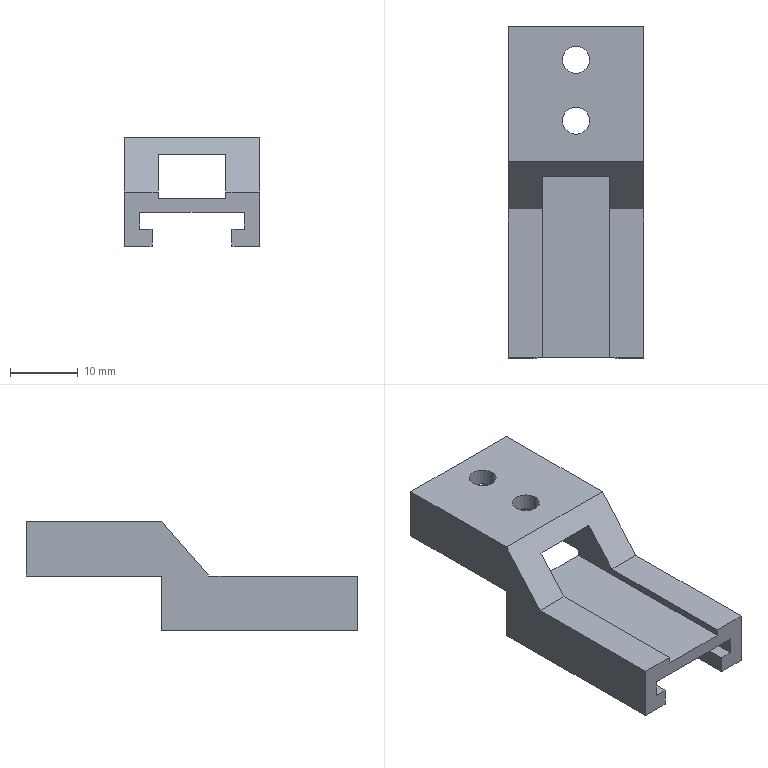Part | 1 solid | 28 faces | box 20 x 49 x 16 mm | volume 4715 mm3 | plane 24 | cylinder 4 | commonest cylinder face diameters 4 x4
STEP:
#1=CARTESIAN_POINT('',(2.,8.5,16.));
#2=VERTEX_POINT('',#1);
#3=CARTESIAN_POINT('',(-2.,8.5,16.));
#4=VERTEX_POINT('',#3);
#5=CARTESIAN_POINT('',(0.,8.5,16.));
#6=DIRECTION('',(0.,0.,-1.));
#7=DIRECTION('',(-1.,0.,0.));
#8=AXIS2_PLACEMENT_3D('',#5,#6,#7);
#9=CIRCLE('',#8,2.);
#10=EDGE_CURVE('',#2,#4,#9,.T.);
#11=ORIENTED_EDGE('',*,*,#10,.F.);
#12=CARTESIAN_POINT('',(2.,8.5,13.5));
#13=VERTEX_POINT('',#12);
#14=CARTESIAN_POINT('',(2.,8.5,45.));
#15=DIRECTION('',(0.,0.,-1.));
#16=VECTOR('',#15,1000.);
#17=LINE('',#14,#16);
#18=EDGE_CURVE('',#2,#13,#17,.T.);
#19=ORIENTED_EDGE('',*,*,#18,.T.);
#20=CARTESIAN_POINT('',(-2.,8.5,13.5));
#21=VERTEX_POINT('',#20);
#22=CARTESIAN_POINT('',(0.,8.5,13.5));
#23=DIRECTION('',(0.,0.,-1.));
#24=DIRECTION('',(1.,0.,0.));
#25=AXIS2_PLACEMENT_3D('',#22,#23,#24);
#26=CIRCLE('',#25,2.);
#27=EDGE_CURVE('',#13,#21,#26,.T.);
#28=ORIENTED_EDGE('',*,*,#27,.T.);
#29=CARTESIAN_POINT('',(-2.,8.5,45.));
#30=DIRECTION('',(0.,0.,-1.));
#31=VECTOR('',#30,1000.);
#32=LINE('',#29,#31);
#33=EDGE_CURVE('',#4,#21,#32,.T.);
#34=ORIENTED_EDGE('',*,*,#33,.F.);
#35=EDGE_LOOP('',(#11,#19,#28,#34));
#36=FACE_OUTER_BOUND('',#35,.T.);
#37=CARTESIAN_POINT('',(0.,8.5,45.));
#38=DIRECTION('',(0.,0.,-1.));
#39=DIRECTION('',(-1.,0.,0.));
#40=AXIS2_PLACEMENT_3D('',#37,#38,#39);
#41=CYLINDRICAL_SURFACE('',#40,2.);
#42=ADVANCED_FACE('',(#36),#41,.F.);
#43=CARTESIAN_POINT('',(2.,17.5,16.));
#44=VERTEX_POINT('',#43);
#45=CARTESIAN_POINT('',(-2.,17.5,16.));
#46=VERTEX_POINT('',#45);
#47=CARTESIAN_POINT('',(0.,17.5,16.));
#48=DIRECTION('',(0.,0.,-1.));
#49=DIRECTION('',(-1.,0.,0.));
#50=AXIS2_PLACEMENT_3D('',#47,#48,#49);
#51=CIRCLE('',#50,2.);
#52=EDGE_CURVE('',#44,#46,#51,.T.);
#53=ORIENTED_EDGE('',*,*,#52,.F.);
#54=CARTESIAN_POINT('',(2.,17.5,13.5));
#55=VERTEX_POINT('',#54);
#56=CARTESIAN_POINT('',(2.,17.5,45.));
#57=DIRECTION('',(0.,0.,-1.));
#58=VECTOR('',#57,1000.);
#59=LINE('',#56,#58);
#60=EDGE_CURVE('',#44,#55,#59,.T.);
#61=ORIENTED_EDGE('',*,*,#60,.T.);
#62=CARTESIAN_POINT('',(-2.,17.5,13.5));
#63=VERTEX_POINT('',#62);
#64=CARTESIAN_POINT('',(0.,17.5,13.5));
#65=DIRECTION('',(0.,0.,-1.));
#66=DIRECTION('',(1.,0.,0.));
#67=AXIS2_PLACEMENT_3D('',#64,#65,#66);
#68=CIRCLE('',#67,2.);
#69=EDGE_CURVE('',#55,#63,#68,.T.);
#70=ORIENTED_EDGE('',*,*,#69,.T.);
#71=CARTESIAN_POINT('',(-2.,17.5,45.));
#72=DIRECTION('',(0.,0.,-1.));
#73=VECTOR('',#72,1000.);
#74=LINE('',#71,#73);
#75=EDGE_CURVE('',#46,#63,#74,.T.);
#76=ORIENTED_EDGE('',*,*,#75,.F.);
#77=EDGE_LOOP('',(#53,#61,#70,#76));
#78=FACE_OUTER_BOUND('',#77,.T.);
#79=CARTESIAN_POINT('',(0.,17.5,45.));
#80=DIRECTION('',(0.,0.,-1.));
#81=DIRECTION('',(-1.,0.,0.));
#82=AXIS2_PLACEMENT_3D('',#79,#80,#81);
#83=CYLINDRICAL_SURFACE('',#82,2.);
#84=ADVANCED_FACE('',(#78),#83,.F.);
#85=CARTESIAN_POINT('',(-5.9,2.5,0.));
#86=VERTEX_POINT('',#85);
#87=CARTESIAN_POINT('',(-5.9,-26.5,0.));
#88=VERTEX_POINT('',#87);
#89=CARTESIAN_POINT('',(-5.9,3.5,0.));
#90=DIRECTION('',(0.,-1.,0.));
#91=VECTOR('',#90,1000.);
#92=LINE('',#89,#91);
#93=EDGE_CURVE('',#86,#88,#92,.T.);
#94=ORIENTED_EDGE('',*,*,#93,.T.);
#95=CARTESIAN_POINT('',(-10.,-26.5,0.));
#96=VERTEX_POINT('',#95);
#97=CARTESIAN_POINT('',(-10.,-26.5,0.));
#98=DIRECTION('',(1.,0.,0.));
#99=VECTOR('',#98,1000.);
#100=LINE('',#97,#99);
#101=EDGE_CURVE('',#96,#88,#100,.T.);
#102=ORIENTED_EDGE('',*,*,#101,.F.);
#103=CARTESIAN_POINT('',(-10.,2.5,0.));
#104=VERTEX_POINT('',#103);
#105=CARTESIAN_POINT('',(-10.,-22.5,0.));
#106=DIRECTION('',(0.,-1.,0.));
#107=VECTOR('',#106,1000.);
#108=LINE('',#105,#107);
#109=EDGE_CURVE('',#104,#96,#108,.T.);
#110=ORIENTED_EDGE('',*,*,#109,.F.);
#111=CARTESIAN_POINT('',(16.,2.5,0.));
#112=DIRECTION('',(-1.,0.,0.));
#113=VECTOR('',#112,1000.);
#114=LINE('',#111,#113);
#115=EDGE_CURVE('',#86,#104,#114,.T.);
#116=ORIENTED_EDGE('',*,*,#115,.F.);
#117=EDGE_LOOP('',(#94,#102,#110,#116));
#118=FACE_OUTER_BOUND('',#117,.T.);
#119=CARTESIAN_POINT('',(0.,0.,0.));
#120=DIRECTION('',(0.,0.,-1.));
#121=DIRECTION('',(-1.,0.,0.));
#122=AXIS2_PLACEMENT_3D('',#119,#120,#121);
#123=PLANE('',#122);
#124=ADVANCED_FACE('',(#118),#123,.T.);
#125=CARTESIAN_POINT('',(10.,2.5,16.));
#126=VERTEX_POINT('',#125);
#127=CARTESIAN_POINT('',(10.,-4.5,8.));
#128=VERTEX_POINT('',#127);
#129=CARTESIAN_POINT('',(10.,-8.341,3.611));
#130=DIRECTION('',(0.,-0.6585,-0.7526));
#131=VECTOR('',#130,1000.);
#132=LINE('',#129,#131);
#133=EDGE_CURVE('',#126,#128,#132,.T.);
#134=ORIENTED_EDGE('',*,*,#133,.T.);
#135=CARTESIAN_POINT('',(10.,-26.5,8.));
#136=VERTEX_POINT('',#135);
#137=CARTESIAN_POINT('',(10.,-22.5,8.));
#138=DIRECTION('',(0.,-1.,0.));
#139=VECTOR('',#138,1000.);
#140=LINE('',#137,#139);
#141=EDGE_CURVE('',#128,#136,#140,.T.);
#142=ORIENTED_EDGE('',*,*,#141,.T.);
#143=CARTESIAN_POINT('',(10.,-26.5,0.));
#144=VERTEX_POINT('',#143);
#145=CARTESIAN_POINT('',(10.,-26.5,0.));
#146=DIRECTION('',(0.,0.,1.));
#147=VECTOR('',#146,1000.);
#148=LINE('',#145,#147);
#149=EDGE_CURVE('',#144,#136,#148,.T.);
#150=ORIENTED_EDGE('',*,*,#149,.F.);
#151=CARTESIAN_POINT('',(10.,2.5,0.));
#152=VERTEX_POINT('',#151);
#153=CARTESIAN_POINT('',(10.,-22.5,0.));
#154=DIRECTION('',(0.,1.,0.));
#155=VECTOR('',#154,1000.);
#156=LINE('',#153,#155);
#157=EDGE_CURVE('',#144,#152,#156,.T.);
#158=ORIENTED_EDGE('',*,*,#157,.T.);
#159=CARTESIAN_POINT('',(10.,2.5,8.));
#160=VERTEX_POINT('',#159);
#161=CARTESIAN_POINT('',(10.,2.5,16.));
#162=DIRECTION('',(0.,0.,1.));
#163=VECTOR('',#162,1000.);
#164=LINE('',#161,#163);
#165=EDGE_CURVE('',#152,#160,#164,.T.);
#166=ORIENTED_EDGE('',*,*,#165,.T.);
#167=CARTESIAN_POINT('',(10.,22.5,8.));
#168=VERTEX_POINT('',#167);
#169=CARTESIAN_POINT('',(10.,-22.5,8.));
#170=DIRECTION('',(0.,1.,0.));
#171=VECTOR('',#170,1000.);
#172=LINE('',#169,#171);
#173=EDGE_CURVE('',#160,#168,#172,.T.);
#174=ORIENTED_EDGE('',*,*,#173,.T.);
#175=CARTESIAN_POINT('',(10.,22.5,16.));
#176=VERTEX_POINT('',#175);
#177=CARTESIAN_POINT('',(10.,22.5,16.));
#178=DIRECTION('',(0.,0.,-1.));
#179=VECTOR('',#178,1000.);
#180=LINE('',#177,#179);
#181=EDGE_CURVE('',#176,#168,#180,.T.);
#182=ORIENTED_EDGE('',*,*,#181,.F.);
#183=CARTESIAN_POINT('',(10.,-22.5,16.));
#184=DIRECTION('',(0.,1.,0.));
#185=VECTOR('',#184,1000.);
#186=LINE('',#183,#185);
#187=EDGE_CURVE('',#126,#176,#186,.T.);
#188=ORIENTED_EDGE('',*,*,#187,.F.);
#189=EDGE_LOOP('',(#134,#142,#150,#158,#166,#174,#182,#188));
#190=FACE_OUTER_BOUND('',#189,.T.);
#191=CARTESIAN_POINT('',(10.,-22.5,16.));
#192=DIRECTION('',(-1.,0.,0.));
#193=DIRECTION('',(0.,0.,1.));
#194=AXIS2_PLACEMENT_3D('',#191,#192,#193);
#195=PLANE('',#194);
#196=ADVANCED_FACE('',(#190),#195,.F.);
#197=ORIENTED_EDGE('',*,*,#181,.T.);
#198=CARTESIAN_POINT('',(5.,22.5,8.));
#199=VERTEX_POINT('',#198);
#200=CARTESIAN_POINT('',(16.,22.5,8.));
#201=DIRECTION('',(-1.,0.,0.));
#202=VECTOR('',#201,1000.);
#203=LINE('',#200,#202);
#204=EDGE_CURVE('',#168,#199,#203,.T.);
#205=ORIENTED_EDGE('',*,*,#204,.T.);
#206=CARTESIAN_POINT('',(5.,22.5,13.5));
#207=VERTEX_POINT('',#206);
#208=CARTESIAN_POINT('',(5.,22.5,7.));
#209=DIRECTION('',(0.,0.,-1.));
#210=VECTOR('',#209,1000.);
#211=LINE('',#208,#210);
#212=EDGE_CURVE('',#207,#199,#211,.T.);
#213=ORIENTED_EDGE('',*,*,#212,.F.);
#214=CARTESIAN_POINT('',(-5.,22.5,13.5));
#215=VERTEX_POINT('',#214);
#216=CARTESIAN_POINT('',(-5.,22.5,13.5));
#217=DIRECTION('',(1.,0.,0.));
#218=VECTOR('',#217,1000.);
#219=LINE('',#216,#218);
#220=EDGE_CURVE('',#215,#207,#219,.T.);
#221=ORIENTED_EDGE('',*,*,#220,.F.);
#222=CARTESIAN_POINT('',(-5.,22.5,8.));
#223=VERTEX_POINT('',#222);
#224=CARTESIAN_POINT('',(-5.,22.5,7.));
#225=DIRECTION('',(0.,0.,1.));
#226=VECTOR('',#225,1000.);
#227=LINE('',#224,#226);
#228=EDGE_CURVE('',#223,#215,#227,.T.);
#229=ORIENTED_EDGE('',*,*,#228,.F.);
#230=CARTESIAN_POINT('',(-10.,22.5,8.));
#231=VERTEX_POINT('',#230);
#232=CARTESIAN_POINT('',(16.,22.5,8.));
#233=DIRECTION('',(-1.,0.,0.));
#234=VECTOR('',#233,1000.);
#235=LINE('',#232,#234);
#236=EDGE_CURVE('',#223,#231,#235,.T.);
#237=ORIENTED_EDGE('',*,*,#236,.T.);
#238=CARTESIAN_POINT('',(-10.,22.5,16.));
#239=VERTEX_POINT('',#238);
#240=CARTESIAN_POINT('',(-10.,22.5,16.));
#241=DIRECTION('',(0.,0.,-1.));
#242=VECTOR('',#241,1000.);
#243=LINE('',#240,#242);
#244=EDGE_CURVE('',#239,#231,#243,.T.);
#245=ORIENTED_EDGE('',*,*,#244,.F.);
#246=CARTESIAN_POINT('',(-10.,22.5,16.));
#247=DIRECTION('',(-1.,0.,0.));
#248=VECTOR('',#247,1000.);
#249=LINE('',#246,#248);
#250=EDGE_CURVE('',#176,#239,#249,.T.);
#251=ORIENTED_EDGE('',*,*,#250,.F.);
#252=EDGE_LOOP('',(#197,#205,#213,#221,#229,#237,#245,#251));
#253=FACE_OUTER_BOUND('',#252,.T.);
#254=CARTESIAN_POINT('',(-10.,22.5,16.));
#255=DIRECTION('',(0.,-1.,0.));
#256=DIRECTION('',(0.,0.,-1.));
#257=AXIS2_PLACEMENT_3D('',#254,#255,#256);
#258=PLANE('',#257);
#259=ADVANCED_FACE('',(#253),#258,.F.);
#260=ORIENTED_EDGE('',*,*,#109,.T.);
#261=CARTESIAN_POINT('',(-10.,-26.5,8.));
#262=VERTEX_POINT('',#261);
#263=CARTESIAN_POINT('',(-10.,-26.5,8.));
#264=DIRECTION('',(0.,0.,-1.));
#265=VECTOR('',#264,1000.);
#266=LINE('',#263,#265);
#267=EDGE_CURVE('',#262,#96,#266,.T.);
#268=ORIENTED_EDGE('',*,*,#267,.F.);
#269=CARTESIAN_POINT('',(-10.,-4.5,8.));
#270=VERTEX_POINT('',#269);
#271=CARTESIAN_POINT('',(-10.,-22.5,8.));
#272=DIRECTION('',(0.,-1.,0.));
#273=VECTOR('',#272,1000.);
#274=LINE('',#271,#273);
#275=EDGE_CURVE('',#270,#262,#274,.T.);
#276=ORIENTED_EDGE('',*,*,#275,.F.);
#277=CARTESIAN_POINT('',(-10.,2.5,16.));
#278=VERTEX_POINT('',#277);
#279=CARTESIAN_POINT('',(-10.,-4.5,8.));
#280=DIRECTION('',(0.,-0.6585,-0.7526));
#281=VECTOR('',#280,1000.);
#282=LINE('',#279,#281);
#283=EDGE_CURVE('',#278,#270,#282,.T.);
#284=ORIENTED_EDGE('',*,*,#283,.F.);
#285=CARTESIAN_POINT('',(-10.,-22.5,16.));
#286=DIRECTION('',(0.,-1.,0.));
#287=VECTOR('',#286,1000.);
#288=LINE('',#285,#287);
#289=EDGE_CURVE('',#239,#278,#288,.T.);
#290=ORIENTED_EDGE('',*,*,#289,.F.);
#291=ORIENTED_EDGE('',*,*,#244,.T.);
#292=CARTESIAN_POINT('',(-10.,2.5,8.));
#293=VERTEX_POINT('',#292);
#294=CARTESIAN_POINT('',(-10.,22.5,8.));
#295=DIRECTION('',(0.,1.,0.));
#296=VECTOR('',#295,1000.);
#297=LINE('',#294,#296);
#298=EDGE_CURVE('',#293,#231,#297,.T.);
#299=ORIENTED_EDGE('',*,*,#298,.F.);
#300=CARTESIAN_POINT('',(-10.,2.5,0.));
#301=DIRECTION('',(0.,0.,1.));
#302=VECTOR('',#301,1000.);
#303=LINE('',#300,#302);
#304=EDGE_CURVE('',#104,#293,#303,.T.);
#305=ORIENTED_EDGE('',*,*,#304,.F.);
#306=EDGE_LOOP('',(#260,#268,#276,#284,#290,#291,#299,#305));
#307=FACE_OUTER_BOUND('',#306,.T.);
#308=CARTESIAN_POINT('',(-10.,-22.5,16.));
#309=DIRECTION('',(1.,0.,0.));
#310=DIRECTION('',(0.,0.,-1.));
#311=AXIS2_PLACEMENT_3D('',#308,#309,#310);
#312=PLANE('',#311);
#313=ADVANCED_FACE('',(#307),#312,.F.);
#314=CARTESIAN_POINT('',(0.,8.5,16.));
#315=DIRECTION('',(0.,0.,-1.));
#316=DIRECTION('',(-1.,0.,0.));
#317=AXIS2_PLACEMENT_3D('',#314,#315,#316);
#318=CIRCLE('',#317,2.);
#319=EDGE_CURVE('',#4,#2,#318,.T.);
#320=ORIENTED_EDGE('',*,*,#319,.T.);
#321=ORIENTED_EDGE('',*,*,#10,.T.);
#322=EDGE_LOOP('',(#320,#321));
#323=FACE_BOUND('',#322,.T.);
#324=CARTESIAN_POINT('',(0.,17.5,16.));
#325=DIRECTION('',(0.,0.,-1.));
#326=DIRECTION('',(-1.,0.,0.));
#327=AXIS2_PLACEMENT_3D('',#324,#325,#326);
#328=CIRCLE('',#327,2.);
#329=EDGE_CURVE('',#46,#44,#328,.T.);
#330=ORIENTED_EDGE('',*,*,#329,.T.);
#331=ORIENTED_EDGE('',*,*,#52,.T.);
#332=EDGE_LOOP('',(#330,#331));
#333=FACE_BOUND('',#332,.T.);
#334=ORIENTED_EDGE('',*,*,#289,.T.);
#335=CARTESIAN_POINT('',(16.,2.5,16.));
#336=DIRECTION('',(-1.,0.,0.));
#337=VECTOR('',#336,1000.);
#338=LINE('',#335,#337);
#339=EDGE_CURVE('',#126,#278,#338,.T.);
#340=ORIENTED_EDGE('',*,*,#339,.F.);
#341=ORIENTED_EDGE('',*,*,#187,.T.);
#342=ORIENTED_EDGE('',*,*,#250,.T.);
#343=EDGE_LOOP('',(#334,#340,#341,#342));
#344=FACE_OUTER_BOUND('',#343,.T.);
#345=CARTESIAN_POINT('',(0.,0.,16.));
#346=DIRECTION('',(0.,0.,-1.));
#347=DIRECTION('',(-1.,0.,0.));
#348=AXIS2_PLACEMENT_3D('',#345,#346,#347);
#349=PLANE('',#348);
#350=ADVANCED_FACE('',(#323,#333,#344),#349,.F.);
#351=CARTESIAN_POINT('',(5.9,2.5,0.));
#352=VERTEX_POINT('',#351);
#353=CARTESIAN_POINT('',(5.9,-26.5,0.));
#354=VERTEX_POINT('',#353);
#355=CARTESIAN_POINT('',(5.9,3.5,0.));
#356=DIRECTION('',(0.,-1.,0.));
#357=VECTOR('',#356,1000.);
#358=LINE('',#355,#357);
#359=EDGE_CURVE('',#352,#354,#358,.T.);
#360=ORIENTED_EDGE('',*,*,#359,.F.);
#361=CARTESIAN_POINT('',(16.,2.5,0.));
#362=DIRECTION('',(-1.,0.,0.));
#363=VECTOR('',#362,1000.);
#364=LINE('',#361,#363);
#365=EDGE_CURVE('',#152,#352,#364,.T.);
#366=ORIENTED_EDGE('',*,*,#365,.F.);
#367=ORIENTED_EDGE('',*,*,#157,.F.);
#368=CARTESIAN_POINT('',(5.9,-26.5,0.));
#369=DIRECTION('',(1.,0.,0.));
#370=VECTOR('',#369,1000.);
#371=LINE('',#368,#370);
#372=EDGE_CURVE('',#354,#144,#371,.T.);
#373=ORIENTED_EDGE('',*,*,#372,.F.);
#374=EDGE_LOOP('',(#360,#366,#367,#373));
#375=FACE_OUTER_BOUND('',#374,.T.);
#376=CARTESIAN_POINT('',(0.,0.,0.));
#377=DIRECTION('',(0.,0.,-1.));
#378=DIRECTION('',(-1.,0.,0.));
#379=AXIS2_PLACEMENT_3D('',#376,#377,#378);
#380=PLANE('',#379);
#381=ADVANCED_FACE('',(#375),#380,.T.);
#382=ORIENTED_EDGE('',*,*,#60,.F.);
#383=ORIENTED_EDGE('',*,*,#329,.F.);
#384=ORIENTED_EDGE('',*,*,#75,.T.);
#385=CARTESIAN_POINT('',(0.,17.5,13.5));
#386=DIRECTION('',(0.,0.,-1.));
#387=DIRECTION('',(1.,0.,0.));
#388=AXIS2_PLACEMENT_3D('',#385,#386,#387);
#389=CIRCLE('',#388,2.);
#390=EDGE_CURVE('',#63,#55,#389,.T.);
#391=ORIENTED_EDGE('',*,*,#390,.T.);
#392=EDGE_LOOP('',(#382,#383,#384,#391));
#393=FACE_OUTER_BOUND('',#392,.T.);
#394=CARTESIAN_POINT('',(0.,17.5,45.));
#395=DIRECTION('',(0.,0.,-1.));
#396=DIRECTION('',(-1.,0.,0.));
#397=AXIS2_PLACEMENT_3D('',#394,#395,#396);
#398=CYLINDRICAL_SURFACE('',#397,2.);
#399=ADVANCED_FACE('',(#393),#398,.F.);
#400=ORIENTED_EDGE('',*,*,#18,.F.);
#401=ORIENTED_EDGE('',*,*,#319,.F.);
#402=ORIENTED_EDGE('',*,*,#33,.T.);
#403=CARTESIAN_POINT('',(0.,8.5,13.5));
#404=DIRECTION('',(0.,0.,-1.));
#405=DIRECTION('',(1.,0.,0.));
#406=AXIS2_PLACEMENT_3D('',#403,#404,#405);
#407=CIRCLE('',#406,2.);
#408=EDGE_CURVE('',#21,#13,#407,.T.);
#409=ORIENTED_EDGE('',*,*,#408,.T.);
#410=EDGE_LOOP('',(#400,#401,#402,#409));
#411=FACE_OUTER_BOUND('',#410,.T.);
#412=CARTESIAN_POINT('',(0.,8.5,45.));
#413=DIRECTION('',(0.,0.,-1.));
#414=DIRECTION('',(-1.,0.,0.));
#415=AXIS2_PLACEMENT_3D('',#412,#413,#414);
#416=CYLINDRICAL_SURFACE('',#415,2.);
#417=ADVANCED_FACE('',(#411),#416,.F.);
#418=CARTESIAN_POINT('',(-5.,0.3125,13.5));
#419=VERTEX_POINT('',#418);
#420=CARTESIAN_POINT('',(-5.,-4.5,8.));
#421=VERTEX_POINT('',#420);
#422=CARTESIAN_POINT('',(-5.,-23.208,-13.381));
#423=DIRECTION('',(0.,-0.6585,-0.7526));
#424=VECTOR('',#423,1000.);
#425=LINE('',#422,#424);
#426=EDGE_CURVE('',#419,#421,#425,.T.);
#427=ORIENTED_EDGE('',*,*,#426,.T.);
#428=CARTESIAN_POINT('',(-5.,-26.5,8.));
#429=VERTEX_POINT('',#428);
#430=CARTESIAN_POINT('',(-5.,-46.5,8.));
#431=DIRECTION('',(0.,-1.,0.));
#432=VECTOR('',#431,1000.);
#433=LINE('',#430,#432);
#434=EDGE_CURVE('',#421,#429,#433,.T.);
#435=ORIENTED_EDGE('',*,*,#434,.T.);
#436=CARTESIAN_POINT('',(-5.,-26.5,7.));
#437=VERTEX_POINT('',#436);
#438=CARTESIAN_POINT('',(-5.,-26.5,7.));
#439=DIRECTION('',(0.,0.,1.));
#440=VECTOR('',#439,1000.);
#441=LINE('',#438,#440);
#442=EDGE_CURVE('',#437,#429,#441,.T.);
#443=ORIENTED_EDGE('',*,*,#442,.F.);
#444=CARTESIAN_POINT('',(-5.,2.5,7.));
#445=VERTEX_POINT('',#444);
#446=CARTESIAN_POINT('',(-5.,-46.5,7.));
#447=DIRECTION('',(0.,1.,0.));
#448=VECTOR('',#447,1000.);
#449=LINE('',#446,#448);
#450=EDGE_CURVE('',#437,#445,#449,.T.);
#451=ORIENTED_EDGE('',*,*,#450,.T.);
#452=CARTESIAN_POINT('',(-5.,2.5,8.));
#453=VERTEX_POINT('',#452);
#454=CARTESIAN_POINT('',(-5.,2.5,7.));
#455=DIRECTION('',(0.,0.,1.));
#456=VECTOR('',#455,1000.);
#457=LINE('',#454,#456);
#458=EDGE_CURVE('',#445,#453,#457,.T.);
#459=ORIENTED_EDGE('',*,*,#458,.T.);
#460=CARTESIAN_POINT('',(-5.,-46.5,8.));
#461=DIRECTION('',(0.,1.,0.));
#462=VECTOR('',#461,1000.);
#463=LINE('',#460,#462);
#464=EDGE_CURVE('',#453,#223,#463,.T.);
#465=ORIENTED_EDGE('',*,*,#464,.T.);
#466=ORIENTED_EDGE('',*,*,#228,.T.);
#467=CARTESIAN_POINT('',(-5.,-46.5,13.5));
#468=DIRECTION('',(0.,1.,0.));
#469=VECTOR('',#468,1000.);
#470=LINE('',#467,#469);
#471=EDGE_CURVE('',#419,#215,#470,.T.);
#472=ORIENTED_EDGE('',*,*,#471,.F.);
#473=EDGE_LOOP('',(#427,#435,#443,#451,#459,#465,#466,#472));
#474=FACE_OUTER_BOUND('',#473,.T.);
#475=CARTESIAN_POINT('',(-5.,-46.5,7.));
#476=DIRECTION('',(-1.,0.,0.));
#477=DIRECTION('',(0.,0.,1.));
#478=AXIS2_PLACEMENT_3D('',#475,#476,#477);
#479=PLANE('',#478);
#480=ADVANCED_FACE('',(#474),#479,.F.);
#481=CARTESIAN_POINT('',(5.,-26.5,7.));
#482=VERTEX_POINT('',#481);
#483=CARTESIAN_POINT('',(5.,2.5,7.));
#484=VERTEX_POINT('',#483);
#485=CARTESIAN_POINT('',(5.,-46.5,7.));
#486=DIRECTION('',(0.,1.,0.));
#487=VECTOR('',#486,1000.);
#488=LINE('',#485,#487);
#489=EDGE_CURVE('',#482,#484,#488,.T.);
#490=ORIENTED_EDGE('',*,*,#489,.F.);
#491=CARTESIAN_POINT('',(5.,-26.5,8.));
#492=VERTEX_POINT('',#491);
#493=CARTESIAN_POINT('',(5.,-26.5,8.));
#494=DIRECTION('',(0.,0.,-1.));
#495=VECTOR('',#494,1000.);
#496=LINE('',#493,#495);
#497=EDGE_CURVE('',#492,#482,#496,.T.);
#498=ORIENTED_EDGE('',*,*,#497,.F.);
#499=CARTESIAN_POINT('',(5.,-4.5,8.));
#500=VERTEX_POINT('',#499);
#501=CARTESIAN_POINT('',(5.,-46.5,8.));
#502=DIRECTION('',(0.,1.,0.));
#503=VECTOR('',#502,1000.);
#504=LINE('',#501,#503);
#505=EDGE_CURVE('',#492,#500,#504,.T.);
#506=ORIENTED_EDGE('',*,*,#505,.T.);
#507=CARTESIAN_POINT('',(5.,0.3125,13.5));
#508=VERTEX_POINT('',#507);
#509=CARTESIAN_POINT('',(5.,-23.208,-13.381));
#510=DIRECTION('',(0.,0.6585,0.7526));
#511=VECTOR('',#510,1000.);
#512=LINE('',#509,#511);
#513=EDGE_CURVE('',#500,#508,#512,.T.);
#514=ORIENTED_EDGE('',*,*,#513,.T.);
#515=CARTESIAN_POINT('',(5.,-46.5,13.5));
#516=DIRECTION('',(0.,1.,0.));
#517=VECTOR('',#516,1000.);
#518=LINE('',#515,#517);
#519=EDGE_CURVE('',#508,#207,#518,.T.);
#520=ORIENTED_EDGE('',*,*,#519,.T.);
#521=ORIENTED_EDGE('',*,*,#212,.T.);
#522=CARTESIAN_POINT('',(5.,2.5,8.));
#523=VERTEX_POINT('',#522);
#524=CARTESIAN_POINT('',(5.,-46.5,8.));
#525=DIRECTION('',(0.,-1.,0.));
#526=VECTOR('',#525,1000.);
#527=LINE('',#524,#526);
#528=EDGE_CURVE('',#199,#523,#527,.T.);
#529=ORIENTED_EDGE('',*,*,#528,.T.);
#530=CARTESIAN_POINT('',(5.,2.5,7.));
#531=DIRECTION('',(0.,0.,-1.));
#532=VECTOR('',#531,1000.);
#533=LINE('',#530,#532);
#534=EDGE_CURVE('',#523,#484,#533,.T.);
#535=ORIENTED_EDGE('',*,*,#534,.T.);
#536=EDGE_LOOP('',(#490,#498,#506,#514,#520,#521,#529,#535));
#537=FACE_OUTER_BOUND('',#536,.T.);
#538=CARTESIAN_POINT('',(5.,-46.5,7.));
#539=DIRECTION('',(1.,0.,0.));
#540=DIRECTION('',(0.,0.,-1.));
#541=AXIS2_PLACEMENT_3D('',#538,#539,#540);
#542=PLANE('',#541);
#543=ADVANCED_FACE('',(#537),#542,.F.);
#544=ORIENTED_EDGE('',*,*,#489,.T.);
#545=CARTESIAN_POINT('',(-5.,2.5,7.));
#546=DIRECTION('',(-1.,0.,0.));
#547=VECTOR('',#546,1000.);
#548=LINE('',#545,#547);
#549=EDGE_CURVE('',#484,#445,#548,.T.);
#550=ORIENTED_EDGE('',*,*,#549,.T.);
#551=ORIENTED_EDGE('',*,*,#450,.F.);
#552=CARTESIAN_POINT('',(5.,-26.5,7.));
#553=DIRECTION('',(-1.,0.,0.));
#554=VECTOR('',#553,1000.);
#555=LINE('',#552,#554);
#556=EDGE_CURVE('',#482,#437,#555,.T.);
#557=ORIENTED_EDGE('',*,*,#556,.F.);
#558=EDGE_LOOP('',(#544,#550,#551,#557));
#559=FACE_OUTER_BOUND('',#558,.T.);
#560=CARTESIAN_POINT('',(-5.,-46.5,7.));
#561=DIRECTION('',(0.,0.,-1.));
#562=DIRECTION('',(-1.,0.,0.));
#563=AXIS2_PLACEMENT_3D('',#560,#561,#562);
#564=PLANE('',#563);
#565=ADVANCED_FACE('',(#559),#564,.F.);
#566=ORIENTED_EDGE('',*,*,#390,.F.);
#567=ORIENTED_EDGE('',*,*,#69,.F.);
#568=EDGE_LOOP('',(#566,#567));
#569=FACE_BOUND('',#568,.T.);
#570=ORIENTED_EDGE('',*,*,#408,.F.);
#571=ORIENTED_EDGE('',*,*,#27,.F.);
#572=EDGE_LOOP('',(#570,#571));
#573=FACE_BOUND('',#572,.T.);
#574=ORIENTED_EDGE('',*,*,#519,.F.);
#575=CARTESIAN_POINT('',(-5.,0.3125,13.5));
#576=DIRECTION('',(-1.,0.,0.));
#577=VECTOR('',#576,1000.);
#578=LINE('',#575,#577);
#579=EDGE_CURVE('',#508,#419,#578,.T.);
#580=ORIENTED_EDGE('',*,*,#579,.T.);
#581=ORIENTED_EDGE('',*,*,#471,.T.);
#582=ORIENTED_EDGE('',*,*,#220,.T.);
#583=EDGE_LOOP('',(#574,#580,#581,#582));
#584=FACE_OUTER_BOUND('',#583,.T.);
#585=CARTESIAN_POINT('',(-5.,-46.5,13.5));
#586=DIRECTION('',(0.,0.,1.));
#587=DIRECTION('',(1.,0.,0.));
#588=AXIS2_PLACEMENT_3D('',#585,#586,#587);
#589=PLANE('',#588);
#590=ADVANCED_FACE('',(#569,#573,#584),#589,.F.);
#591=CARTESIAN_POINT('',(16.,2.5,8.));
#592=DIRECTION('',(-1.,0.,0.));
#593=VECTOR('',#592,1000.);
#594=LINE('',#591,#593);
#595=EDGE_CURVE('',#160,#523,#594,.T.);
#596=ORIENTED_EDGE('',*,*,#595,.T.);
#597=ORIENTED_EDGE('',*,*,#528,.F.);
#598=ORIENTED_EDGE('',*,*,#204,.F.);
#599=ORIENTED_EDGE('',*,*,#173,.F.);
#600=EDGE_LOOP('',(#596,#597,#598,#599));
#601=FACE_OUTER_BOUND('',#600,.T.);
#602=CARTESIAN_POINT('',(16.,22.5,8.));
#603=DIRECTION('',(0.,0.,1.));
#604=DIRECTION('',(0.,-1.,0.));
#605=AXIS2_PLACEMENT_3D('',#602,#603,#604);
#606=PLANE('',#605);
#607=ADVANCED_FACE('',(#601),#606,.F.);
#608=CARTESIAN_POINT('',(16.,2.5,8.));
#609=DIRECTION('',(-1.,0.,0.));
#610=VECTOR('',#609,1000.);
#611=LINE('',#608,#610);
#612=EDGE_CURVE('',#453,#293,#611,.T.);
#613=ORIENTED_EDGE('',*,*,#612,.T.);
#614=ORIENTED_EDGE('',*,*,#298,.T.);
#615=ORIENTED_EDGE('',*,*,#236,.F.);
#616=ORIENTED_EDGE('',*,*,#464,.F.);
#617=EDGE_LOOP('',(#613,#614,#615,#616));
#618=FACE_OUTER_BOUND('',#617,.T.);
#619=CARTESIAN_POINT('',(16.,22.5,8.));
#620=DIRECTION('',(0.,0.,1.));
#621=DIRECTION('',(0.,-1.,0.));
#622=AXIS2_PLACEMENT_3D('',#619,#620,#621);
#623=PLANE('',#622);
#624=ADVANCED_FACE('',(#618),#623,.F.);
#625=CARTESIAN_POINT('',(-7.75,2.5,2.5));
#626=VERTEX_POINT('',#625);
#627=CARTESIAN_POINT('',(-5.9,2.5,2.5));
#628=VERTEX_POINT('',#627);
#629=CARTESIAN_POINT('',(16.,2.5,2.5));
#630=DIRECTION('',(1.,0.,0.));
#631=VECTOR('',#630,1000.);
#632=LINE('',#629,#631);
#633=EDGE_CURVE('',#626,#628,#632,.T.);
#634=ORIENTED_EDGE('',*,*,#633,.T.);
#635=CARTESIAN_POINT('',(-5.9,2.5,0.));
#636=DIRECTION('',(0.,0.,-1.));
#637=VECTOR('',#636,1000.);
#638=LINE('',#635,#637);
#639=EDGE_CURVE('',#628,#86,#638,.T.);
#640=ORIENTED_EDGE('',*,*,#639,.T.);
#641=ORIENTED_EDGE('',*,*,#115,.T.);
#642=ORIENTED_EDGE('',*,*,#304,.T.);
#643=ORIENTED_EDGE('',*,*,#612,.F.);
#644=ORIENTED_EDGE('',*,*,#458,.F.);
#645=ORIENTED_EDGE('',*,*,#549,.F.);
#646=ORIENTED_EDGE('',*,*,#534,.F.);
#647=ORIENTED_EDGE('',*,*,#595,.F.);
#648=ORIENTED_EDGE('',*,*,#165,.F.);
#649=ORIENTED_EDGE('',*,*,#365,.T.);
#650=CARTESIAN_POINT('',(5.9,2.5,2.5));
#651=VERTEX_POINT('',#650);
#652=CARTESIAN_POINT('',(5.9,2.5,0.));
#653=DIRECTION('',(0.,0.,1.));
#654=VECTOR('',#653,1000.);
#655=LINE('',#652,#654);
#656=EDGE_CURVE('',#352,#651,#655,.T.);
#657=ORIENTED_EDGE('',*,*,#656,.T.);
#658=CARTESIAN_POINT('',(7.75,2.5,2.5));
#659=VERTEX_POINT('',#658);
#660=CARTESIAN_POINT('',(16.,2.5,2.5));
#661=DIRECTION('',(1.,0.,0.));
#662=VECTOR('',#661,1000.);
#663=LINE('',#660,#662);
#664=EDGE_CURVE('',#651,#659,#663,.T.);
#665=ORIENTED_EDGE('',*,*,#664,.T.);
#666=CARTESIAN_POINT('',(7.75,2.5,5.));
#667=VERTEX_POINT('',#666);
#668=CARTESIAN_POINT('',(7.75,2.5,0.));
#669=DIRECTION('',(0.,0.,1.));
#670=VECTOR('',#669,1000.);
#671=LINE('',#668,#670);
#672=EDGE_CURVE('',#659,#667,#671,.T.);
#673=ORIENTED_EDGE('',*,*,#672,.T.);
#674=CARTESIAN_POINT('',(-7.75,2.5,5.));
#675=VERTEX_POINT('',#674);
#676=CARTESIAN_POINT('',(16.,2.5,5.));
#677=DIRECTION('',(-1.,0.,0.));
#678=VECTOR('',#677,1000.);
#679=LINE('',#676,#678);
#680=EDGE_CURVE('',#667,#675,#679,.T.);
#681=ORIENTED_EDGE('',*,*,#680,.T.);
#682=CARTESIAN_POINT('',(-7.75,2.5,0.));
#683=DIRECTION('',(0.,0.,-1.));
#684=VECTOR('',#683,1000.);
#685=LINE('',#682,#684);
#686=EDGE_CURVE('',#675,#626,#685,.T.);
#687=ORIENTED_EDGE('',*,*,#686,.T.);
#688=EDGE_LOOP('',(#634,#640,#641,#642,#643,#644,#645,#646,#647,#648,#649,#657,#665,#673,#681,#687));
#689=FACE_OUTER_BOUND('',#688,.T.);
#690=CARTESIAN_POINT('',(16.,2.5,0.));
#691=DIRECTION('',(0.,-1.,0.));
#692=DIRECTION('',(0.,0.,-1.));
#693=AXIS2_PLACEMENT_3D('',#690,#691,#692);
#694=PLANE('',#693);
#695=ADVANCED_FACE('',(#689),#694,.F.);
#696=CARTESIAN_POINT('',(16.,-4.5,8.));
#697=DIRECTION('',(-1.,0.,0.));
#698=VECTOR('',#697,1000.);
#699=LINE('',#696,#698);
#700=EDGE_CURVE('',#128,#500,#699,.T.);
#701=ORIENTED_EDGE('',*,*,#700,.T.);
#702=ORIENTED_EDGE('',*,*,#505,.F.);
#703=CARTESIAN_POINT('',(10.,-26.5,8.));
#704=DIRECTION('',(-1.,0.,0.));
#705=VECTOR('',#704,1000.);
#706=LINE('',#703,#705);
#707=EDGE_CURVE('',#136,#492,#706,.T.);
#708=ORIENTED_EDGE('',*,*,#707,.F.);
#709=ORIENTED_EDGE('',*,*,#141,.F.);
#710=EDGE_LOOP('',(#701,#702,#708,#709));
#711=FACE_OUTER_BOUND('',#710,.T.);
#712=CARTESIAN_POINT('',(16.,-22.5,8.));
#713=DIRECTION('',(0.,0.,-1.));
#714=DIRECTION('',(-1.,0.,0.));
#715=AXIS2_PLACEMENT_3D('',#712,#713,#714);
#716=PLANE('',#715);
#717=ADVANCED_FACE('',(#711),#716,.F.);
#718=CARTESIAN_POINT('',(16.,-4.5,8.));
#719=DIRECTION('',(-1.,0.,0.));
#720=VECTOR('',#719,1000.);
#721=LINE('',#718,#720);
#722=EDGE_CURVE('',#421,#270,#721,.T.);
#723=ORIENTED_EDGE('',*,*,#722,.T.);
#724=ORIENTED_EDGE('',*,*,#275,.T.);
#725=CARTESIAN_POINT('',(-5.,-26.5,8.));
#726=DIRECTION('',(-1.,0.,0.));
#727=VECTOR('',#726,1000.);
#728=LINE('',#725,#727);
#729=EDGE_CURVE('',#429,#262,#728,.T.);
#730=ORIENTED_EDGE('',*,*,#729,.F.);
#731=ORIENTED_EDGE('',*,*,#434,.F.);
#732=EDGE_LOOP('',(#723,#724,#730,#731));
#733=FACE_OUTER_BOUND('',#732,.T.);
#734=CARTESIAN_POINT('',(16.,-22.5,8.));
#735=DIRECTION('',(0.,0.,-1.));
#736=DIRECTION('',(-1.,0.,0.));
#737=AXIS2_PLACEMENT_3D('',#734,#735,#736);
#738=PLANE('',#737);
#739=ADVANCED_FACE('',(#733),#738,.F.);
#740=ORIENTED_EDGE('',*,*,#339,.T.);
#741=ORIENTED_EDGE('',*,*,#283,.T.);
#742=ORIENTED_EDGE('',*,*,#722,.F.);
#743=ORIENTED_EDGE('',*,*,#426,.F.);
#744=ORIENTED_EDGE('',*,*,#579,.F.);
#745=ORIENTED_EDGE('',*,*,#513,.F.);
#746=ORIENTED_EDGE('',*,*,#700,.F.);
#747=ORIENTED_EDGE('',*,*,#133,.F.);
#748=EDGE_LOOP('',(#740,#741,#742,#743,#744,#745,#746,#747));
#749=FACE_OUTER_BOUND('',#748,.T.);
#750=CARTESIAN_POINT('',(16.,-4.5,8.));
#751=DIRECTION('',(0.,0.7526,-0.6585));
#752=DIRECTION('',(0.,0.6585,0.7526));
#753=AXIS2_PLACEMENT_3D('',#750,#751,#752);
#754=PLANE('',#753);
#755=ADVANCED_FACE('',(#749),#754,.F.);
#756=CARTESIAN_POINT('',(-5.9,-26.5,2.5));
#757=VERTEX_POINT('',#756);
#758=CARTESIAN_POINT('',(-5.9,3.5,2.5));
#759=DIRECTION('',(0.,-1.,0.));
#760=VECTOR('',#759,1000.);
#761=LINE('',#758,#760);
#762=EDGE_CURVE('',#628,#757,#761,.T.);
#763=ORIENTED_EDGE('',*,*,#762,.T.);
#764=CARTESIAN_POINT('',(-5.9,-26.5,0.));
#765=DIRECTION('',(0.,0.,1.));
#766=VECTOR('',#765,1000.);
#767=LINE('',#764,#766);
#768=EDGE_CURVE('',#88,#757,#767,.T.);
#769=ORIENTED_EDGE('',*,*,#768,.F.);
#770=ORIENTED_EDGE('',*,*,#93,.F.);
#771=ORIENTED_EDGE('',*,*,#639,.F.);
#772=EDGE_LOOP('',(#763,#769,#770,#771));
#773=FACE_OUTER_BOUND('',#772,.T.);
#774=CARTESIAN_POINT('',(-5.9,3.5,0.));
#775=DIRECTION('',(-1.,0.,0.));
#776=DIRECTION('',(0.,0.,1.));
#777=AXIS2_PLACEMENT_3D('',#774,#775,#776);
#778=PLANE('',#777);
#779=ADVANCED_FACE('',(#773),#778,.F.);
#780=CARTESIAN_POINT('',(-7.75,-26.5,2.5));
#781=VERTEX_POINT('',#780);
#782=CARTESIAN_POINT('',(-7.75,3.5,2.5));
#783=DIRECTION('',(0.,-1.,0.));
#784=VECTOR('',#783,1000.);
#785=LINE('',#782,#784);
#786=EDGE_CURVE('',#626,#781,#785,.T.);
#787=ORIENTED_EDGE('',*,*,#786,.T.);
#788=CARTESIAN_POINT('',(-5.9,-26.5,2.5));
#789=DIRECTION('',(-1.,0.,0.));
#790=VECTOR('',#789,1000.);
#791=LINE('',#788,#790);
#792=EDGE_CURVE('',#757,#781,#791,.T.);
#793=ORIENTED_EDGE('',*,*,#792,.F.);
#794=ORIENTED_EDGE('',*,*,#762,.F.);
#795=ORIENTED_EDGE('',*,*,#633,.F.);
#796=EDGE_LOOP('',(#787,#793,#794,#795));
#797=FACE_OUTER_BOUND('',#796,.T.);
#798=CARTESIAN_POINT('',(-5.9,3.5,2.5));
#799=DIRECTION('',(0.,0.,-1.));
#800=DIRECTION('',(-1.,0.,0.));
#801=AXIS2_PLACEMENT_3D('',#798,#799,#800);
#802=PLANE('',#801);
#803=ADVANCED_FACE('',(#797),#802,.F.);
#804=CARTESIAN_POINT('',(-7.75,-26.5,5.));
#805=VERTEX_POINT('',#804);
#806=CARTESIAN_POINT('',(-7.75,3.5,5.));
#807=DIRECTION('',(0.,-1.,0.));
#808=VECTOR('',#807,1000.);
#809=LINE('',#806,#808);
#810=EDGE_CURVE('',#675,#805,#809,.T.);
#811=ORIENTED_EDGE('',*,*,#810,.T.);
#812=CARTESIAN_POINT('',(-7.75,-26.5,2.5));
#813=DIRECTION('',(0.,0.,1.));
#814=VECTOR('',#813,1000.);
#815=LINE('',#812,#814);
#816=EDGE_CURVE('',#781,#805,#815,.T.);
#817=ORIENTED_EDGE('',*,*,#816,.F.);
#818=ORIENTED_EDGE('',*,*,#786,.F.);
#819=ORIENTED_EDGE('',*,*,#686,.F.);
#820=EDGE_LOOP('',(#811,#817,#818,#819));
#821=FACE_OUTER_BOUND('',#820,.T.);
#822=CARTESIAN_POINT('',(-7.75,3.5,2.5));
#823=DIRECTION('',(-1.,0.,0.));
#824=DIRECTION('',(0.,0.,1.));
#825=AXIS2_PLACEMENT_3D('',#822,#823,#824);
#826=PLANE('',#825);
#827=ADVANCED_FACE('',(#821),#826,.F.);
#828=CARTESIAN_POINT('',(7.75,-26.5,5.));
#829=VERTEX_POINT('',#828);
#830=CARTESIAN_POINT('',(7.75,3.5,5.));
#831=DIRECTION('',(0.,-1.,0.));
#832=VECTOR('',#831,1000.);
#833=LINE('',#830,#832);
#834=EDGE_CURVE('',#667,#829,#833,.T.);
#835=ORIENTED_EDGE('',*,*,#834,.T.);
#836=CARTESIAN_POINT('',(-7.75,-26.5,5.));
#837=DIRECTION('',(1.,0.,0.));
#838=VECTOR('',#837,1000.);
#839=LINE('',#836,#838);
#840=EDGE_CURVE('',#805,#829,#839,.T.);
#841=ORIENTED_EDGE('',*,*,#840,.F.);
#842=ORIENTED_EDGE('',*,*,#810,.F.);
#843=ORIENTED_EDGE('',*,*,#680,.F.);
#844=EDGE_LOOP('',(#835,#841,#842,#843));
#845=FACE_OUTER_BOUND('',#844,.T.);
#846=CARTESIAN_POINT('',(-7.75,3.5,5.));
#847=DIRECTION('',(0.,0.,1.));
#848=DIRECTION('',(1.,0.,0.));
#849=AXIS2_PLACEMENT_3D('',#846,#847,#848);
#850=PLANE('',#849);
#851=ADVANCED_FACE('',(#845),#850,.F.);
#852=CARTESIAN_POINT('',(7.75,-26.5,2.5));
#853=VERTEX_POINT('',#852);
#854=CARTESIAN_POINT('',(7.75,3.5,2.5));
#855=DIRECTION('',(0.,-1.,0.));
#856=VECTOR('',#855,1000.);
#857=LINE('',#854,#856);
#858=EDGE_CURVE('',#659,#853,#857,.T.);
#859=ORIENTED_EDGE('',*,*,#858,.T.);
#860=CARTESIAN_POINT('',(7.75,-26.5,5.));
#861=DIRECTION('',(0.,0.,-1.));
#862=VECTOR('',#861,1000.);
#863=LINE('',#860,#862);
#864=EDGE_CURVE('',#829,#853,#863,.T.);
#865=ORIENTED_EDGE('',*,*,#864,.F.);
#866=ORIENTED_EDGE('',*,*,#834,.F.);
#867=ORIENTED_EDGE('',*,*,#672,.F.);
#868=EDGE_LOOP('',(#859,#865,#866,#867));
#869=FACE_OUTER_BOUND('',#868,.T.);
#870=CARTESIAN_POINT('',(7.75,3.5,2.5));
#871=DIRECTION('',(1.,0.,0.));
#872=DIRECTION('',(0.,0.,-1.));
#873=AXIS2_PLACEMENT_3D('',#870,#871,#872);
#874=PLANE('',#873);
#875=ADVANCED_FACE('',(#869),#874,.F.);
#876=CARTESIAN_POINT('',(5.9,-26.5,2.5));
#877=VERTEX_POINT('',#876);
#878=CARTESIAN_POINT('',(5.9,3.5,2.5));
#879=DIRECTION('',(0.,-1.,0.));
#880=VECTOR('',#879,1000.);
#881=LINE('',#878,#880);
#882=EDGE_CURVE('',#651,#877,#881,.T.);
#883=ORIENTED_EDGE('',*,*,#882,.T.);
#884=CARTESIAN_POINT('',(7.75,-26.5,2.5));
#885=DIRECTION('',(-1.,0.,0.));
#886=VECTOR('',#885,1000.);
#887=LINE('',#884,#886);
#888=EDGE_CURVE('',#853,#877,#887,.T.);
#889=ORIENTED_EDGE('',*,*,#888,.F.);
#890=ORIENTED_EDGE('',*,*,#858,.F.);
#891=ORIENTED_EDGE('',*,*,#664,.F.);
#892=EDGE_LOOP('',(#883,#889,#890,#891));
#893=FACE_OUTER_BOUND('',#892,.T.);
#894=CARTESIAN_POINT('',(5.9,3.5,2.5));
#895=DIRECTION('',(0.,0.,-1.));
#896=DIRECTION('',(-1.,0.,0.));
#897=AXIS2_PLACEMENT_3D('',#894,#895,#896);
#898=PLANE('',#897);
#899=ADVANCED_FACE('',(#893),#898,.F.);
#900=ORIENTED_EDGE('',*,*,#359,.T.);
#901=CARTESIAN_POINT('',(5.9,-26.5,2.5));
#902=DIRECTION('',(0.,0.,-1.));
#903=VECTOR('',#902,1000.);
#904=LINE('',#901,#903);
#905=EDGE_CURVE('',#877,#354,#904,.T.);
#906=ORIENTED_EDGE('',*,*,#905,.F.);
#907=ORIENTED_EDGE('',*,*,#882,.F.);
#908=ORIENTED_EDGE('',*,*,#656,.F.);
#909=EDGE_LOOP('',(#900,#906,#907,#908));
#910=FACE_OUTER_BOUND('',#909,.T.);
#911=CARTESIAN_POINT('',(5.9,3.5,0.));
#912=DIRECTION('',(1.,0.,0.));
#913=DIRECTION('',(0.,0.,-1.));
#914=AXIS2_PLACEMENT_3D('',#911,#912,#913);
#915=PLANE('',#914);
#916=ADVANCED_FACE('',(#910),#915,.F.);
#917=ORIENTED_EDGE('',*,*,#267,.T.);
#918=ORIENTED_EDGE('',*,*,#101,.T.);
#919=ORIENTED_EDGE('',*,*,#768,.T.);
#920=ORIENTED_EDGE('',*,*,#792,.T.);
#921=ORIENTED_EDGE('',*,*,#816,.T.);
#922=ORIENTED_EDGE('',*,*,#840,.T.);
#923=ORIENTED_EDGE('',*,*,#864,.T.);
#924=ORIENTED_EDGE('',*,*,#888,.T.);
#925=ORIENTED_EDGE('',*,*,#905,.T.);
#926=ORIENTED_EDGE('',*,*,#372,.T.);
#927=ORIENTED_EDGE('',*,*,#149,.T.);
#928=ORIENTED_EDGE('',*,*,#707,.T.);
#929=ORIENTED_EDGE('',*,*,#497,.T.);
#930=ORIENTED_EDGE('',*,*,#556,.T.);
#931=ORIENTED_EDGE('',*,*,#442,.T.);
#932=ORIENTED_EDGE('',*,*,#729,.T.);
#933=EDGE_LOOP('',(#917,#918,#919,#920,#921,#922,#923,#924,#925,#926,#927,#928,#929,#930,#931,#932));
#934=FACE_OUTER_BOUND('',#933,.T.);
#935=CARTESIAN_POINT('',(0.,-26.5,0.));
#936=DIRECTION('',(0.,-1.,0.));
#937=DIRECTION('',(0.,0.,-1.));
#938=AXIS2_PLACEMENT_3D('',#935,#936,#937);
#939=PLANE('',#938);
#940=ADVANCED_FACE('',(#934),#939,.T.);
#941=CLOSED_SHELL('',(#42,#84,#124,#196,#259,#313,#350,#381,#399,#417,#480,#543,#565,#590,#607,#624,#695,#717,#739,#755,#779,#803,#827,#851,#875,#899,#916,#940));
#942=MANIFOLD_SOLID_BREP('',#941);
#943=CARTESIAN_POINT('',(0.,0.,0.));
#944=DIRECTION('',(0.,0.,1.));
#945=DIRECTION('',(1.,0.,0.));
#946=AXIS2_PLACEMENT_3D('',#943,#944,#945);
#947=(LENGTH_UNIT()NAMED_UNIT(*)SI_UNIT(.MILLI.,.METRE.));
#948=UNCERTAINTY_MEASURE_WITH_UNIT(LENGTH_MEASURE(0.00001),#947,'','');
#949=(NAMED_UNIT(*)PLANE_ANGLE_UNIT()SI_UNIT($,.RADIAN.));
#950=(NAMED_UNIT(*)SI_UNIT($,.STERADIAN.)SOLID_ANGLE_UNIT());
#951=(GEOMETRIC_REPRESENTATION_CONTEXT(3)GLOBAL_UNCERTAINTY_ASSIGNED_CONTEXT((#948))GLOBAL_UNIT_ASSIGNED_CONTEXT((#947,#949,#950))REPRESENTATION_CONTEXT('',''));
#952=ADVANCED_BREP_SHAPE_REPRESENTATION('',(#942,#946),#951);